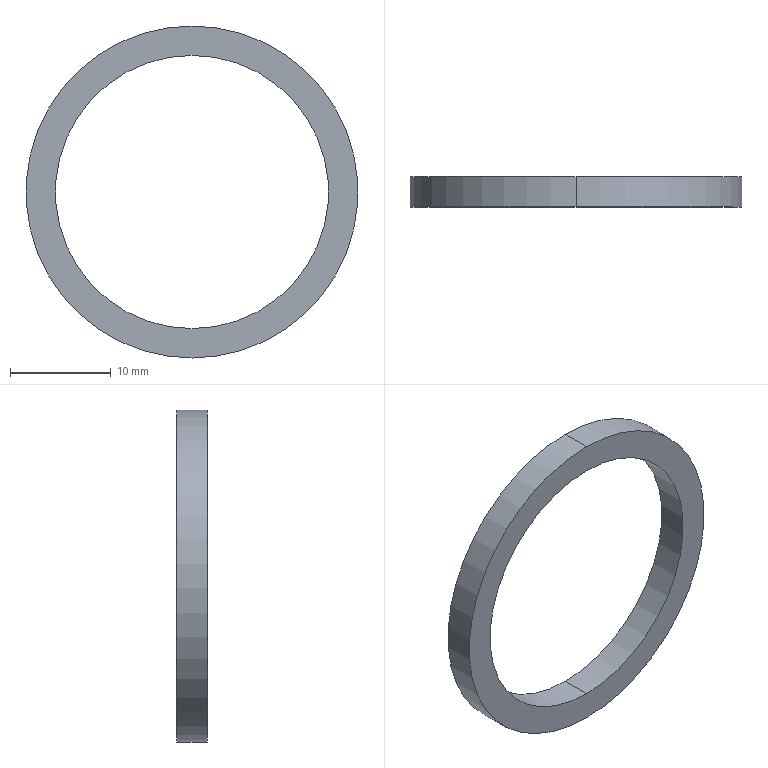Part | SolidWorks | features Extrusion 1 | 1 solid | 6 faces | box 33 x 3 x 33 mm | volume 829.092 mm3 | cylinder 4 | plane 2 | commonest cylinder face diameters 27.15 x2 33 x2
STEP:
#1=CARTESIAN_POINT('',(0.,3.,-13.575));
#2=VERTEX_POINT('',#1);
#3=CARTESIAN_POINT('',(0.,3.,13.575));
#4=VERTEX_POINT('',#3);
#5=CARTESIAN_POINT('',(0.,3.,0.));
#6=DIRECTION('',(0.,1.,0.));
#7=DIRECTION('',(0.,0.,1.));
#8=AXIS2_PLACEMENT_3D('',#5,#6,#7);
#9=CIRCLE('',#8,13.575);
#10=EDGE_CURVE('',#2,#4,#9,.T.);
#11=ORIENTED_EDGE('',*,*,#10,.T.);
#12=CARTESIAN_POINT('',(0.,0.,13.575));
#13=VERTEX_POINT('',#12);
#14=CARTESIAN_POINT('',(0.,3.,13.575));
#15=DIRECTION('',(0.,-1.,0.));
#16=VECTOR('',#15,1000.);
#17=LINE('',#14,#16);
#18=EDGE_CURVE('',#4,#13,#17,.T.);
#19=ORIENTED_EDGE('',*,*,#18,.T.);
#20=CARTESIAN_POINT('',(0.,0.,-13.575));
#21=VERTEX_POINT('',#20);
#22=CARTESIAN_POINT('',(0.,0.,0.));
#23=DIRECTION('',(0.,1.,0.));
#24=DIRECTION('',(0.,0.,1.));
#25=AXIS2_PLACEMENT_3D('',#22,#23,#24);
#26=CIRCLE('',#25,13.575);
#27=EDGE_CURVE('',#21,#13,#26,.T.);
#28=ORIENTED_EDGE('',*,*,#27,.F.);
#29=CARTESIAN_POINT('',(0.,3.,-13.575));
#30=DIRECTION('',(0.,-1.,0.));
#31=VECTOR('',#30,1000.);
#32=LINE('',#29,#31);
#33=EDGE_CURVE('',#2,#21,#32,.T.);
#34=ORIENTED_EDGE('',*,*,#33,.F.);
#35=EDGE_LOOP('',(#11,#19,#28,#34));
#36=FACE_OUTER_BOUND('',#35,.T.);
#37=CARTESIAN_POINT('',(0.,3.,0.));
#38=DIRECTION('',(0.,-1.,0.));
#39=DIRECTION('',(0.,0.,-1.));
#40=AXIS2_PLACEMENT_3D('',#37,#38,#39);
#41=CYLINDRICAL_SURFACE('',#40,13.575);
#42=ADVANCED_FACE('',(#36),#41,.F.);
#43=CARTESIAN_POINT('',(0.,3.,16.5));
#44=VERTEX_POINT('',#43);
#45=CARTESIAN_POINT('',(0.,3.,-16.5));
#46=VERTEX_POINT('',#45);
#47=CARTESIAN_POINT('',(0.,3.,0.));
#48=DIRECTION('',(0.,1.,0.));
#49=DIRECTION('',(0.,0.,1.));
#50=AXIS2_PLACEMENT_3D('',#47,#48,#49);
#51=CIRCLE('',#50,16.5);
#52=EDGE_CURVE('',#44,#46,#51,.T.);
#53=ORIENTED_EDGE('',*,*,#52,.F.);
#54=CARTESIAN_POINT('',(0.,0.,16.5));
#55=VERTEX_POINT('',#54);
#56=CARTESIAN_POINT('',(0.,3.,16.5));
#57=DIRECTION('',(0.,-1.,0.));
#58=VECTOR('',#57,1000.);
#59=LINE('',#56,#58);
#60=EDGE_CURVE('',#44,#55,#59,.T.);
#61=ORIENTED_EDGE('',*,*,#60,.T.);
#62=CARTESIAN_POINT('',(0.,0.,-16.5));
#63=VERTEX_POINT('',#62);
#64=CARTESIAN_POINT('',(0.,0.,0.));
#65=DIRECTION('',(0.,1.,0.));
#66=DIRECTION('',(0.,0.,1.));
#67=AXIS2_PLACEMENT_3D('',#64,#65,#66);
#68=CIRCLE('',#67,16.5);
#69=EDGE_CURVE('',#55,#63,#68,.T.);
#70=ORIENTED_EDGE('',*,*,#69,.T.);
#71=CARTESIAN_POINT('',(0.,3.,-16.5));
#72=DIRECTION('',(0.,-1.,0.));
#73=VECTOR('',#72,1000.);
#74=LINE('',#71,#73);
#75=EDGE_CURVE('',#46,#63,#74,.T.);
#76=ORIENTED_EDGE('',*,*,#75,.F.);
#77=EDGE_LOOP('',(#53,#61,#70,#76));
#78=FACE_OUTER_BOUND('',#77,.T.);
#79=CARTESIAN_POINT('',(0.,3.,0.));
#80=DIRECTION('',(0.,-1.,0.));
#81=DIRECTION('',(0.,0.,-1.));
#82=AXIS2_PLACEMENT_3D('',#79,#80,#81);
#83=CYLINDRICAL_SURFACE('',#82,16.5);
#84=ADVANCED_FACE('',(#78),#83,.T.);
#85=CARTESIAN_POINT('',(0.,3.,0.));
#86=DIRECTION('',(0.,1.,0.));
#87=DIRECTION('',(0.,0.,1.));
#88=AXIS2_PLACEMENT_3D('',#85,#86,#87);
#89=CIRCLE('',#88,16.5);
#90=EDGE_CURVE('',#46,#44,#89,.T.);
#91=ORIENTED_EDGE('',*,*,#90,.T.);
#92=ORIENTED_EDGE('',*,*,#52,.T.);
#93=EDGE_LOOP('',(#91,#92));
#94=FACE_OUTER_BOUND('',#93,.T.);
#95=ORIENTED_EDGE('',*,*,#10,.F.);
#96=CARTESIAN_POINT('',(0.,3.,0.));
#97=DIRECTION('',(0.,1.,0.));
#98=DIRECTION('',(0.,0.,1.));
#99=AXIS2_PLACEMENT_3D('',#96,#97,#98);
#100=CIRCLE('',#99,13.575);
#101=EDGE_CURVE('',#4,#2,#100,.T.);
#102=ORIENTED_EDGE('',*,*,#101,.F.);
#103=EDGE_LOOP('',(#95,#102));
#104=FACE_BOUND('',#103,.T.);
#105=CARTESIAN_POINT('',(0.,3.,0.));
#106=DIRECTION('',(0.,1.,0.));
#107=DIRECTION('',(0.,0.,1.));
#108=AXIS2_PLACEMENT_3D('',#105,#106,#107);
#109=PLANE('',#108);
#110=ADVANCED_FACE('',(#94,#104),#109,.T.);
#111=CARTESIAN_POINT('',(0.,0.,0.));
#112=DIRECTION('',(0.,1.,0.));
#113=DIRECTION('',(0.,0.,1.));
#114=AXIS2_PLACEMENT_3D('',#111,#112,#113);
#115=CIRCLE('',#114,16.5);
#116=EDGE_CURVE('',#63,#55,#115,.T.);
#117=ORIENTED_EDGE('',*,*,#116,.F.);
#118=ORIENTED_EDGE('',*,*,#69,.F.);
#119=EDGE_LOOP('',(#117,#118));
#120=FACE_OUTER_BOUND('',#119,.T.);
#121=ORIENTED_EDGE('',*,*,#27,.T.);
#122=CARTESIAN_POINT('',(0.,0.,0.));
#123=DIRECTION('',(0.,1.,0.));
#124=DIRECTION('',(0.,0.,1.));
#125=AXIS2_PLACEMENT_3D('',#122,#123,#124);
#126=CIRCLE('',#125,13.575);
#127=EDGE_CURVE('',#13,#21,#126,.T.);
#128=ORIENTED_EDGE('',*,*,#127,.T.);
#129=EDGE_LOOP('',(#121,#128));
#130=FACE_BOUND('',#129,.T.);
#131=CARTESIAN_POINT('',(0.,0.,0.));
#132=DIRECTION('',(0.,1.,0.));
#133=DIRECTION('',(0.,0.,1.));
#134=AXIS2_PLACEMENT_3D('',#131,#132,#133);
#135=PLANE('',#134);
#136=ADVANCED_FACE('',(#120,#130),#135,.F.);
#137=ORIENTED_EDGE('',*,*,#60,.F.);
#138=ORIENTED_EDGE('',*,*,#90,.F.);
#139=ORIENTED_EDGE('',*,*,#75,.T.);
#140=ORIENTED_EDGE('',*,*,#116,.T.);
#141=EDGE_LOOP('',(#137,#138,#139,#140));
#142=FACE_OUTER_BOUND('',#141,.T.);
#143=CARTESIAN_POINT('',(0.,3.,0.));
#144=DIRECTION('',(0.,-1.,0.));
#145=DIRECTION('',(0.,0.,-1.));
#146=AXIS2_PLACEMENT_3D('',#143,#144,#145);
#147=CYLINDRICAL_SURFACE('',#146,16.5);
#148=ADVANCED_FACE('',(#142),#147,.T.);
#149=ORIENTED_EDGE('',*,*,#18,.F.);
#150=ORIENTED_EDGE('',*,*,#101,.T.);
#151=ORIENTED_EDGE('',*,*,#33,.T.);
#152=ORIENTED_EDGE('',*,*,#127,.F.);
#153=EDGE_LOOP('',(#149,#150,#151,#152));
#154=FACE_OUTER_BOUND('',#153,.T.);
#155=CARTESIAN_POINT('',(0.,3.,0.));
#156=DIRECTION('',(0.,-1.,0.));
#157=DIRECTION('',(0.,0.,-1.));
#158=AXIS2_PLACEMENT_3D('',#155,#156,#157);
#159=CYLINDRICAL_SURFACE('',#158,13.575);
#160=ADVANCED_FACE('',(#154),#159,.F.);
#161=CLOSED_SHELL('',(#42,#84,#110,#136,#148,#160));
#162=MANIFOLD_SOLID_BREP('',#161);
#163=CARTESIAN_POINT('',(0.,0.,0.));
#164=DIRECTION('',(0.,0.,1.));
#165=DIRECTION('',(1.,0.,0.));
#166=AXIS2_PLACEMENT_3D('',#163,#164,#165);
#167=(LENGTH_UNIT()NAMED_UNIT(*)SI_UNIT(.MILLI.,.METRE.));
#168=UNCERTAINTY_MEASURE_WITH_UNIT(LENGTH_MEASURE(0.00001),#167,'','');
#169=(NAMED_UNIT(*)PLANE_ANGLE_UNIT()SI_UNIT($,.RADIAN.));
#170=(NAMED_UNIT(*)SI_UNIT($,.STERADIAN.)SOLID_ANGLE_UNIT());
#171=(GEOMETRIC_REPRESENTATION_CONTEXT(3)GLOBAL_UNCERTAINTY_ASSIGNED_CONTEXT((#168))GLOBAL_UNIT_ASSIGNED_CONTEXT((#167,#169,#170))REPRESENTATION_CONTEXT('',''));
#172=ADVANCED_BREP_SHAPE_REPRESENTATION('',(#162,#166),#171);